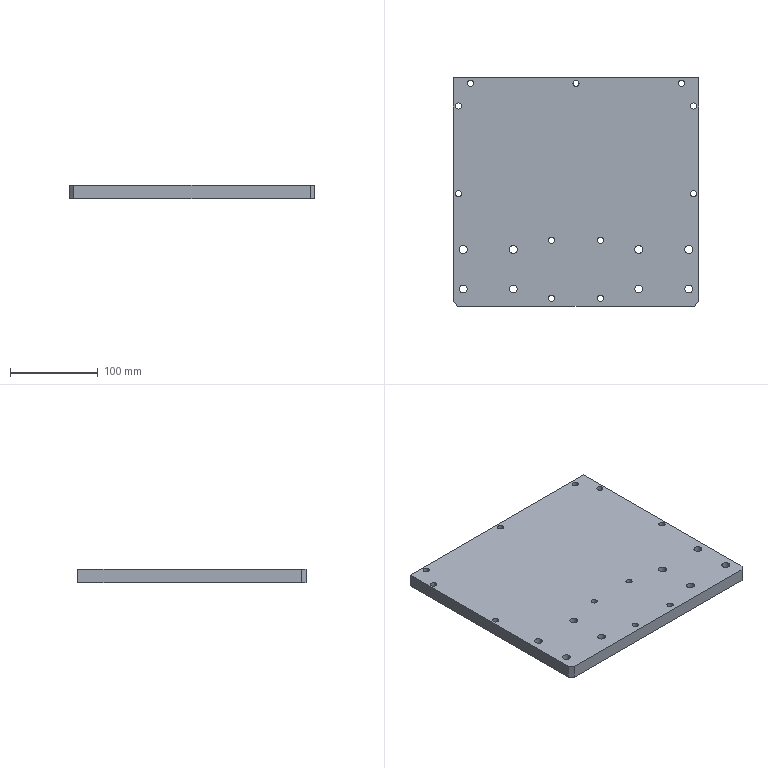Part | SolidWorks | features HoleWzd 4, Chamfer 1, Extrusion 1 | 1 solid | 46 faces | box 280 x 260 x 15 mm | volume 1077641 mm3 | cylinder 38 | plane 8 | commonest cylinder face diameters 7 x22 9 x16